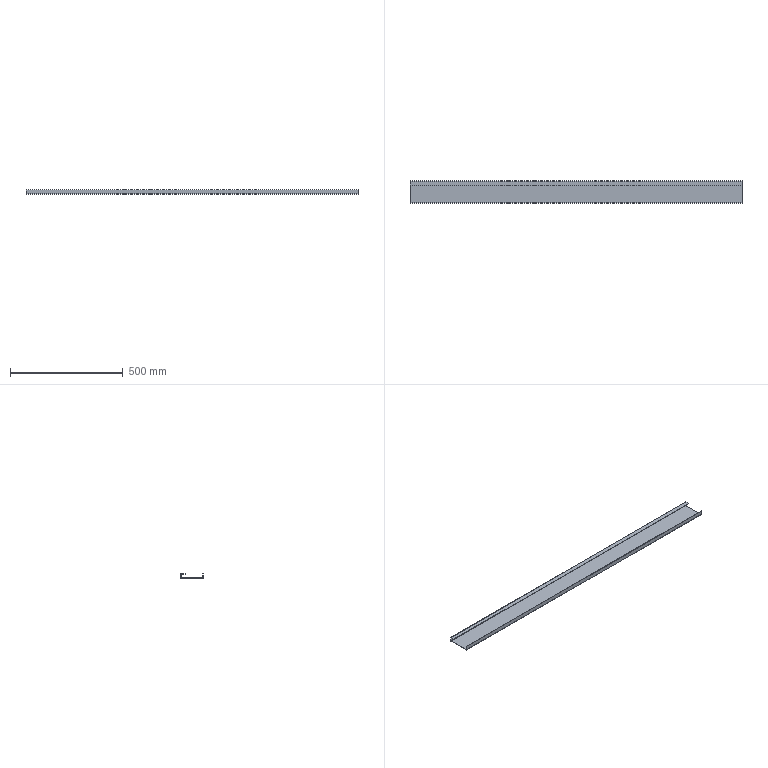Part | STEP file | 粉仓楼梯通道踢脚Plate 2 | 1 solid | 18 faces | box 1470 x 100 x 20 mm | volume 337909 mm3 | plane 12 | cylinder 6 | commonest cylinder face diameters 2 x3 5 x3
STEP:
#1=CARTESIAN_POINT('',(0.,0.,0.));
#2=DIRECTION('',(0.,0.,1.));
#3=DIRECTION('',(1.,0.,0.));
#4=AXIS2_PLACEMENT_3D('',#1,#2,#3);
#5=CARTESIAN_POINT('',(-735.,1.5,2.5));
#6=VERTEX_POINT('',#5);
#7=CARTESIAN_POINT('',(-735.,1.5,20.));
#8=VERTEX_POINT('',#7);
#9=CARTESIAN_POINT('',(-735.,1.5,2.5));
#10=DIRECTION('',(0.,0.,1.));
#11=VECTOR('',#10,1.);
#12=LINE('',#9,#11);
#13=CARTESIAN_POINT('',(735.,1.5,2.5));
#14=DIRECTION('',(0.,-1.,0.));
#15=DIRECTION('',(0.,0.,-1.));
#16=AXIS2_PLACEMENT_3D('',#13,#14,#15);
#17=PLANE('',#16);
#18=CARTESIAN_POINT('',(0.,-1470.));
#19=DIRECTION('',(-1.,0.));
#20=VECTOR('',#19,1.);
#21=LINE('',#18,#20);
#22=(GEOMETRIC_REPRESENTATION_CONTEXT(2)PARAMETRIC_REPRESENTATION_CONTEXT()REPRESENTATION_CONTEXT('',''));
#23=DEFINITIONAL_REPRESENTATION('',(#21),#22);
#24=PCURVE('',#17,#23);
#25=CARTESIAN_POINT('',(-735.,2.5,2.5));
#26=DIRECTION('',(-1.,0.,0.));
#27=DIRECTION('',(0.,0.,1.));
#28=AXIS2_PLACEMENT_3D('',#25,#26,#27);
#29=PLANE('',#28);
#30=CARTESIAN_POINT('',(0.,-1.));
#31=DIRECTION('',(1.,0.));
#32=VECTOR('',#31,1.);
#33=LINE('',#30,#32);
#34=(GEOMETRIC_REPRESENTATION_CONTEXT(2)PARAMETRIC_REPRESENTATION_CONTEXT()REPRESENTATION_CONTEXT('',''));
#35=DEFINITIONAL_REPRESENTATION('',(#33),#34);
#36=PCURVE('',#29,#35);
#37=SURFACE_CURVE('',#12,(#24,#36),.PCURVE_S1.);
#38=EDGE_CURVE('',#6,#8,#37,.T.);
#39=ORIENTED_EDGE('',*,*,#38,.T.);
#40=CARTESIAN_POINT('',(735.,1.5,20.));
#41=VERTEX_POINT('',#40);
#42=CARTESIAN_POINT('',(735.,1.5,20.));
#43=DIRECTION('',(-1.,0.,0.));
#44=VECTOR('',#43,1.);
#45=LINE('',#42,#44);
#46=CARTESIAN_POINT('',(-17.5,0.));
#47=DIRECTION('',(0.,-1.));
#48=VECTOR('',#47,1.);
#49=LINE('',#46,#48);
#50=(GEOMETRIC_REPRESENTATION_CONTEXT(2)PARAMETRIC_REPRESENTATION_CONTEXT()REPRESENTATION_CONTEXT('',''));
#51=DEFINITIONAL_REPRESENTATION('',(#49),#50);
#52=PCURVE('',#17,#51);
#53=CARTESIAN_POINT('',(735.,0.,20.));
#54=DIRECTION('',(0.,0.,1.));
#55=DIRECTION('',(1.,0.,0.));
#56=AXIS2_PLACEMENT_3D('',#53,#54,#55);
#57=PLANE('',#56);
#58=CARTESIAN_POINT('',(0.,1.5));
#59=DIRECTION('',(-1.,0.));
#60=VECTOR('',#59,1.);
#61=LINE('',#58,#60);
#62=(GEOMETRIC_REPRESENTATION_CONTEXT(2)PARAMETRIC_REPRESENTATION_CONTEXT()REPRESENTATION_CONTEXT('',''));
#63=DEFINITIONAL_REPRESENTATION('',(#61),#62);
#64=PCURVE('',#57,#63);
#65=SURFACE_CURVE('',#45,(#52,#64),.PCURVE_S1.);
#66=EDGE_CURVE('',#41,#8,#65,.T.);
#67=ORIENTED_EDGE('',*,*,#66,.F.);
#68=CARTESIAN_POINT('',(735.,1.5,2.5));
#69=VERTEX_POINT('',#68);
#70=CARTESIAN_POINT('',(735.,1.5,2.5));
#71=DIRECTION('',(0.,0.,1.));
#72=VECTOR('',#71,1.);
#73=LINE('',#70,#72);
#74=CARTESIAN_POINT('',(0.,0.));
#75=DIRECTION('',(-1.,0.));
#76=VECTOR('',#75,1.);
#77=LINE('',#74,#76);
#78=(GEOMETRIC_REPRESENTATION_CONTEXT(2)PARAMETRIC_REPRESENTATION_CONTEXT()REPRESENTATION_CONTEXT('',''));
#79=DEFINITIONAL_REPRESENTATION('',(#77),#78);
#80=PCURVE('',#17,#79);
#81=CARTESIAN_POINT('',(735.,2.5,2.5));
#82=DIRECTION('',(-1.,0.,0.));
#83=DIRECTION('',(0.,0.,1.));
#84=AXIS2_PLACEMENT_3D('',#81,#82,#83);
#85=PLANE('',#84);
#86=CARTESIAN_POINT('',(0.,-1.));
#87=DIRECTION('',(1.,0.));
#88=VECTOR('',#87,1.);
#89=LINE('',#86,#88);
#90=(GEOMETRIC_REPRESENTATION_CONTEXT(2)PARAMETRIC_REPRESENTATION_CONTEXT()REPRESENTATION_CONTEXT('',''));
#91=DEFINITIONAL_REPRESENTATION('',(#89),#90);
#92=PCURVE('',#85,#91);
#93=SURFACE_CURVE('',#73,(#80,#92),.PCURVE_S1.);
#94=EDGE_CURVE('',#69,#41,#93,.T.);
#95=ORIENTED_EDGE('',*,*,#94,.F.);
#96=CARTESIAN_POINT('',(735.,1.5,2.5));
#97=DIRECTION('',(-1.,0.,0.));
#98=VECTOR('',#97,1.);
#99=LINE('',#96,#98);
#100=CARTESIAN_POINT('',(0.,0.));
#101=DIRECTION('',(0.,-1.));
#102=VECTOR('',#101,1.);
#103=LINE('',#100,#102);
#104=(GEOMETRIC_REPRESENTATION_CONTEXT(2)PARAMETRIC_REPRESENTATION_CONTEXT()REPRESENTATION_CONTEXT('',''));
#105=DEFINITIONAL_REPRESENTATION('',(#103),#104);
#106=PCURVE('',#17,#105);
#107=CARTESIAN_POINT('',(735.,2.5,2.5));
#108=DIRECTION('',(-1.,0.,0.));
#109=DIRECTION('',(0.,0.,1.));
#110=AXIS2_PLACEMENT_3D('',#107,#108,#109);
#111=CYLINDRICAL_SURFACE('',#110,1.);
#112=CARTESIAN_POINT('',(4.712,0.));
#113=DIRECTION('',(0.,1.));
#114=VECTOR('',#113,1.);
#115=LINE('',#112,#114);
#116=(GEOMETRIC_REPRESENTATION_CONTEXT(2)PARAMETRIC_REPRESENTATION_CONTEXT()REPRESENTATION_CONTEXT('',''));
#117=DEFINITIONAL_REPRESENTATION('',(#115),#116);
#118=PCURVE('',#111,#117);
#119=SURFACE_CURVE('',#99,(#106,#118),.PCURVE_S1.);
#120=EDGE_CURVE('',#69,#6,#119,.T.);
#121=ORIENTED_EDGE('',*,*,#120,.T.);
#122=EDGE_LOOP('',(#39,#67,#95,#121));
#123=FACE_BOUND('',#122,.T.);
#124=ADVANCED_FACE('',(#123),#17,.F.);
#125=CARTESIAN_POINT('',(-735.,0.,20.));
#126=VERTEX_POINT('',#125);
#127=CARTESIAN_POINT('',(-735.,0.,20.));
#128=DIRECTION('',(0.,1.,0.));
#129=VECTOR('',#128,1.);
#130=LINE('',#127,#129);
#131=CARTESIAN_POINT('',(-1470.,0.));
#132=DIRECTION('',(0.,1.));
#133=VECTOR('',#132,1.);
#134=LINE('',#131,#133);
#135=(GEOMETRIC_REPRESENTATION_CONTEXT(2)PARAMETRIC_REPRESENTATION_CONTEXT()REPRESENTATION_CONTEXT('',''));
#136=DEFINITIONAL_REPRESENTATION('',(#134),#135);
#137=PCURVE('',#57,#136);
#138=CARTESIAN_POINT('',(17.5,-2.5));
#139=DIRECTION('',(0.,1.));
#140=VECTOR('',#139,1.);
#141=LINE('',#138,#140);
#142=(GEOMETRIC_REPRESENTATION_CONTEXT(2)PARAMETRIC_REPRESENTATION_CONTEXT()REPRESENTATION_CONTEXT('',''));
#143=DEFINITIONAL_REPRESENTATION('',(#141),#142);
#144=PCURVE('',#29,#143);
#145=SURFACE_CURVE('',#130,(#137,#144),.PCURVE_S1.);
#146=EDGE_CURVE('',#126,#8,#145,.T.);
#147=ORIENTED_EDGE('',*,*,#146,.F.);
#148=CARTESIAN_POINT('',(735.,0.,20.));
#149=VERTEX_POINT('',#148);
#150=CARTESIAN_POINT('',(735.,0.,20.));
#151=DIRECTION('',(-1.,0.,0.));
#152=VECTOR('',#151,1.);
#153=LINE('',#150,#152);
#154=CARTESIAN_POINT('',(0.,0.));
#155=DIRECTION('',(-1.,0.));
#156=VECTOR('',#155,1.);
#157=LINE('',#154,#156);
#158=(GEOMETRIC_REPRESENTATION_CONTEXT(2)PARAMETRIC_REPRESENTATION_CONTEXT()REPRESENTATION_CONTEXT('',''));
#159=DEFINITIONAL_REPRESENTATION('',(#157),#158);
#160=PCURVE('',#57,#159);
#161=CARTESIAN_POINT('',(735.,0.,2.5));
#162=DIRECTION('',(0.,-1.,0.));
#163=DIRECTION('',(0.,0.,-1.));
#164=AXIS2_PLACEMENT_3D('',#161,#162,#163);
#165=PLANE('',#164);
#166=CARTESIAN_POINT('',(-17.5,0.));
#167=DIRECTION('',(0.,-1.));
#168=VECTOR('',#167,1.);
#169=LINE('',#166,#168);
#170=(GEOMETRIC_REPRESENTATION_CONTEXT(2)PARAMETRIC_REPRESENTATION_CONTEXT()REPRESENTATION_CONTEXT('',''));
#171=DEFINITIONAL_REPRESENTATION('',(#169),#170);
#172=PCURVE('',#165,#171);
#173=SURFACE_CURVE('',#153,(#160,#172),.PCURVE_S1.);
#174=EDGE_CURVE('',#149,#126,#173,.T.);
#175=ORIENTED_EDGE('',*,*,#174,.F.);
#176=CARTESIAN_POINT('',(735.,0.,20.));
#177=DIRECTION('',(0.,1.,0.));
#178=VECTOR('',#177,1.);
#179=LINE('',#176,#178);
#180=CARTESIAN_POINT('',(0.,0.));
#181=DIRECTION('',(0.,1.));
#182=VECTOR('',#181,1.);
#183=LINE('',#180,#182);
#184=(GEOMETRIC_REPRESENTATION_CONTEXT(2)PARAMETRIC_REPRESENTATION_CONTEXT()REPRESENTATION_CONTEXT('',''));
#185=DEFINITIONAL_REPRESENTATION('',(#183),#184);
#186=PCURVE('',#57,#185);
#187=CARTESIAN_POINT('',(17.5,-2.5));
#188=DIRECTION('',(0.,1.));
#189=VECTOR('',#188,1.);
#190=LINE('',#187,#189);
#191=(GEOMETRIC_REPRESENTATION_CONTEXT(2)PARAMETRIC_REPRESENTATION_CONTEXT()REPRESENTATION_CONTEXT('',''));
#192=DEFINITIONAL_REPRESENTATION('',(#190),#191);
#193=PCURVE('',#85,#192);
#194=SURFACE_CURVE('',#179,(#186,#193),.PCURVE_S1.);
#195=EDGE_CURVE('',#149,#41,#194,.T.);
#196=ORIENTED_EDGE('',*,*,#195,.T.);
#197=ORIENTED_EDGE('',*,*,#66,.T.);
#198=EDGE_LOOP('',(#147,#175,#196,#197));
#199=FACE_BOUND('',#198,.T.);
#200=ADVANCED_FACE('',(#199),#57,.T.);
#201=CARTESIAN_POINT('',(-735.,0.,2.5));
#202=VERTEX_POINT('',#201);
#203=CARTESIAN_POINT('',(-735.,0.,2.5));
#204=DIRECTION('',(0.,0.,1.));
#205=VECTOR('',#204,1.);
#206=LINE('',#203,#205);
#207=CARTESIAN_POINT('',(0.,-1470.));
#208=DIRECTION('',(-1.,0.));
#209=VECTOR('',#208,1.);
#210=LINE('',#207,#209);
#211=(GEOMETRIC_REPRESENTATION_CONTEXT(2)PARAMETRIC_REPRESENTATION_CONTEXT()REPRESENTATION_CONTEXT('',''));
#212=DEFINITIONAL_REPRESENTATION('',(#210),#211);
#213=PCURVE('',#165,#212);
#214=CARTESIAN_POINT('',(0.,-2.5));
#215=DIRECTION('',(1.,0.));
#216=VECTOR('',#215,1.);
#217=LINE('',#214,#216);
#218=(GEOMETRIC_REPRESENTATION_CONTEXT(2)PARAMETRIC_REPRESENTATION_CONTEXT()REPRESENTATION_CONTEXT('',''));
#219=DEFINITIONAL_REPRESENTATION('',(#217),#218);
#220=PCURVE('',#29,#219);
#221=SURFACE_CURVE('',#206,(#213,#220),.PCURVE_S1.);
#222=EDGE_CURVE('',#202,#126,#221,.T.);
#223=ORIENTED_EDGE('',*,*,#222,.F.);
#224=CARTESIAN_POINT('',(735.,0.,2.5));
#225=VERTEX_POINT('',#224);
#226=CARTESIAN_POINT('',(735.,0.,2.5));
#227=DIRECTION('',(-1.,0.,0.));
#228=VECTOR('',#227,1.);
#229=LINE('',#226,#228);
#230=CARTESIAN_POINT('',(0.,0.));
#231=DIRECTION('',(0.,-1.));
#232=VECTOR('',#231,1.);
#233=LINE('',#230,#232);
#234=(GEOMETRIC_REPRESENTATION_CONTEXT(2)PARAMETRIC_REPRESENTATION_CONTEXT()REPRESENTATION_CONTEXT('',''));
#235=DEFINITIONAL_REPRESENTATION('',(#233),#234);
#236=PCURVE('',#165,#235);
#237=CARTESIAN_POINT('',(735.,2.5,2.5));
#238=DIRECTION('',(-1.,0.,0.));
#239=DIRECTION('',(0.,0.,1.));
#240=AXIS2_PLACEMENT_3D('',#237,#238,#239);
#241=CYLINDRICAL_SURFACE('',#240,2.5);
#242=CARTESIAN_POINT('',(4.712,0.));
#243=DIRECTION('',(0.,1.));
#244=VECTOR('',#243,1.);
#245=LINE('',#242,#244);
#246=(GEOMETRIC_REPRESENTATION_CONTEXT(2)PARAMETRIC_REPRESENTATION_CONTEXT()REPRESENTATION_CONTEXT('',''));
#247=DEFINITIONAL_REPRESENTATION('',(#245),#246);
#248=PCURVE('',#241,#247);
#249=SURFACE_CURVE('',#229,(#236,#248),.PCURVE_S1.);
#250=EDGE_CURVE('',#225,#202,#249,.T.);
#251=ORIENTED_EDGE('',*,*,#250,.F.);
#252=CARTESIAN_POINT('',(735.,0.,2.5));
#253=DIRECTION('',(0.,0.,1.));
#254=VECTOR('',#253,1.);
#255=LINE('',#252,#254);
#256=CARTESIAN_POINT('',(0.,0.));
#257=DIRECTION('',(-1.,0.));
#258=VECTOR('',#257,1.);
#259=LINE('',#256,#258);
#260=(GEOMETRIC_REPRESENTATION_CONTEXT(2)PARAMETRIC_REPRESENTATION_CONTEXT()REPRESENTATION_CONTEXT('',''));
#261=DEFINITIONAL_REPRESENTATION('',(#259),#260);
#262=PCURVE('',#165,#261);
#263=CARTESIAN_POINT('',(0.,-2.5));
#264=DIRECTION('',(1.,0.));
#265=VECTOR('',#264,1.);
#266=LINE('',#263,#265);
#267=(GEOMETRIC_REPRESENTATION_CONTEXT(2)PARAMETRIC_REPRESENTATION_CONTEXT()REPRESENTATION_CONTEXT('',''));
#268=DEFINITIONAL_REPRESENTATION('',(#266),#267);
#269=PCURVE('',#85,#268);
#270=SURFACE_CURVE('',#255,(#262,#269),.PCURVE_S1.);
#271=EDGE_CURVE('',#225,#149,#270,.T.);
#272=ORIENTED_EDGE('',*,*,#271,.T.);
#273=ORIENTED_EDGE('',*,*,#174,.T.);
#274=EDGE_LOOP('',(#223,#251,#272,#273));
#275=FACE_BOUND('',#274,.T.);
#276=ADVANCED_FACE('',(#275),#165,.T.);
#277=CARTESIAN_POINT('',(-735.,2.5,0.));
#278=VERTEX_POINT('',#277);
#279=CARTESIAN_POINT('',(-735.,2.5,2.5));
#280=DIRECTION('',(-1.,0.,0.));
#281=DIRECTION('',(0.,0.,1.));
#282=AXIS2_PLACEMENT_3D('',#279,#280,#281);
#283=CIRCLE('',#282,2.5);
#284=CARTESIAN_POINT('',(0.,1470.));
#285=DIRECTION('',(1.,0.));
#286=VECTOR('',#285,1.);
#287=LINE('',#284,#286);
#288=(GEOMETRIC_REPRESENTATION_CONTEXT(2)PARAMETRIC_REPRESENTATION_CONTEXT()REPRESENTATION_CONTEXT('',''));
#289=DEFINITIONAL_REPRESENTATION('',(#287),#288);
#290=PCURVE('',#241,#289);
#291=CARTESIAN_POINT('',(0.,0.));
#292=DIRECTION('',(1.,0.));
#293=AXIS2_PLACEMENT_2D('',#291,#292);
#294=CIRCLE('',#293,2.5);
#295=(GEOMETRIC_REPRESENTATION_CONTEXT(2)PARAMETRIC_REPRESENTATION_CONTEXT()REPRESENTATION_CONTEXT('',''));
#296=DEFINITIONAL_REPRESENTATION('',(#294),#295);
#297=PCURVE('',#29,#296);
#298=SURFACE_CURVE('',#283,(#290,#297),.PCURVE_S1.);
#299=EDGE_CURVE('',#278,#202,#298,.T.);
#300=ORIENTED_EDGE('',*,*,#299,.F.);
#301=CARTESIAN_POINT('',(735.,2.5,0.));
#302=VERTEX_POINT('',#301);
#303=CARTESIAN_POINT('',(735.,2.5,0.));
#304=DIRECTION('',(-1.,0.,0.));
#305=VECTOR('',#304,1.);
#306=LINE('',#303,#305);
#307=CARTESIAN_POINT('',(3.142,0.));
#308=DIRECTION('',(0.,1.));
#309=VECTOR('',#308,1.);
#310=LINE('',#307,#309);
#311=(GEOMETRIC_REPRESENTATION_CONTEXT(2)PARAMETRIC_REPRESENTATION_CONTEXT()REPRESENTATION_CONTEXT('',''));
#312=DEFINITIONAL_REPRESENTATION('',(#310),#311);
#313=PCURVE('',#241,#312);
#314=CARTESIAN_POINT('',(735.,2.5,0.));
#315=DIRECTION('',(0.,0.,-1.));
#316=DIRECTION('',(-1.,0.,0.));
#317=AXIS2_PLACEMENT_3D('',#314,#315,#316);
#318=PLANE('',#317);
#319=CARTESIAN_POINT('',(0.,0.));
#320=DIRECTION('',(1.,0.));
#321=VECTOR('',#320,1.);
#322=LINE('',#319,#321);
#323=(GEOMETRIC_REPRESENTATION_CONTEXT(2)PARAMETRIC_REPRESENTATION_CONTEXT()REPRESENTATION_CONTEXT('',''));
#324=DEFINITIONAL_REPRESENTATION('',(#322),#323);
#325=PCURVE('',#318,#324);
#326=SURFACE_CURVE('',#306,(#313,#325),.PCURVE_S1.);
#327=EDGE_CURVE('',#302,#278,#326,.T.);
#328=ORIENTED_EDGE('',*,*,#327,.F.);
#329=CARTESIAN_POINT('',(735.,2.5,2.5));
#330=DIRECTION('',(-1.,0.,0.));
#331=DIRECTION('',(0.,0.,1.));
#332=AXIS2_PLACEMENT_3D('',#329,#330,#331);
#333=CIRCLE('',#332,2.5);
#334=CARTESIAN_POINT('',(0.,0.));
#335=DIRECTION('',(1.,0.));
#336=VECTOR('',#335,1.);
#337=LINE('',#334,#336);
#338=(GEOMETRIC_REPRESENTATION_CONTEXT(2)PARAMETRIC_REPRESENTATION_CONTEXT()REPRESENTATION_CONTEXT('',''));
#339=DEFINITIONAL_REPRESENTATION('',(#337),#338);
#340=PCURVE('',#241,#339);
#341=CARTESIAN_POINT('',(0.,0.));
#342=DIRECTION('',(1.,0.));
#343=AXIS2_PLACEMENT_2D('',#341,#342);
#344=CIRCLE('',#343,2.5);
#345=(GEOMETRIC_REPRESENTATION_CONTEXT(2)PARAMETRIC_REPRESENTATION_CONTEXT()REPRESENTATION_CONTEXT('',''));
#346=DEFINITIONAL_REPRESENTATION('',(#344),#345);
#347=PCURVE('',#85,#346);
#348=SURFACE_CURVE('',#333,(#340,#347),.PCURVE_S1.);
#349=EDGE_CURVE('',#302,#225,#348,.T.);
#350=ORIENTED_EDGE('',*,*,#349,.T.);
#351=ORIENTED_EDGE('',*,*,#250,.T.);
#352=EDGE_LOOP('',(#300,#328,#350,#351));
#353=FACE_BOUND('',#352,.T.);
#354=ADVANCED_FACE('',(#353),#241,.T.);
#355=CARTESIAN_POINT('',(-735.,97.5,0.));
#356=VERTEX_POINT('',#355);
#357=CARTESIAN_POINT('',(-735.,2.5,0.));
#358=DIRECTION('',(0.,-1.,0.));
#359=VECTOR('',#358,1.);
#360=LINE('',#357,#359);
#361=CARTESIAN_POINT('',(1470.,0.));
#362=DIRECTION('',(0.,-1.));
#363=VECTOR('',#362,1.);
#364=LINE('',#361,#363);
#365=(GEOMETRIC_REPRESENTATION_CONTEXT(2)PARAMETRIC_REPRESENTATION_CONTEXT()REPRESENTATION_CONTEXT('',''));
#366=DEFINITIONAL_REPRESENTATION('',(#364),#365);
#367=PCURVE('',#318,#366);
#368=CARTESIAN_POINT('',(-2.5,0.));
#369=DIRECTION('',(0.,-1.));
#370=VECTOR('',#369,1.);
#371=LINE('',#368,#370);
#372=(GEOMETRIC_REPRESENTATION_CONTEXT(2)PARAMETRIC_REPRESENTATION_CONTEXT()REPRESENTATION_CONTEXT('',''));
#373=DEFINITIONAL_REPRESENTATION('',(#371),#372);
#374=PCURVE('',#29,#373);
#375=SURFACE_CURVE('',#360,(#367,#374),.PCURVE_S1.);
#376=EDGE_CURVE('',#356,#278,#375,.T.);
#377=ORIENTED_EDGE('',*,*,#376,.F.);
#378=CARTESIAN_POINT('',(735.,97.5,0.));
#379=VERTEX_POINT('',#378);
#380=CARTESIAN_POINT('',(735.,97.5,0.));
#381=DIRECTION('',(-1.,0.,0.));
#382=VECTOR('',#381,1.);
#383=LINE('',#380,#382);
#384=CARTESIAN_POINT('',(0.,95.));
#385=DIRECTION('',(1.,0.));
#386=VECTOR('',#385,1.);
#387=LINE('',#384,#386);
#388=(GEOMETRIC_REPRESENTATION_CONTEXT(2)PARAMETRIC_REPRESENTATION_CONTEXT()REPRESENTATION_CONTEXT('',''));
#389=DEFINITIONAL_REPRESENTATION('',(#387),#388);
#390=PCURVE('',#318,#389);
#391=CARTESIAN_POINT('',(735.,97.5,2.5));
#392=DIRECTION('',(-1.,0.,0.));
#393=DIRECTION('',(0.,0.,1.));
#394=AXIS2_PLACEMENT_3D('',#391,#392,#393);
#395=CYLINDRICAL_SURFACE('',#394,2.5);
#396=CARTESIAN_POINT('',(3.142,0.));
#397=DIRECTION('',(0.,1.));
#398=VECTOR('',#397,1.);
#399=LINE('',#396,#398);
#400=(GEOMETRIC_REPRESENTATION_CONTEXT(2)PARAMETRIC_REPRESENTATION_CONTEXT()REPRESENTATION_CONTEXT('',''));
#401=DEFINITIONAL_REPRESENTATION('',(#399),#400);
#402=PCURVE('',#395,#401);
#403=SURFACE_CURVE('',#383,(#390,#402),.PCURVE_S1.);
#404=EDGE_CURVE('',#379,#356,#403,.T.);
#405=ORIENTED_EDGE('',*,*,#404,.F.);
#406=CARTESIAN_POINT('',(735.,2.5,0.));
#407=DIRECTION('',(0.,-1.,0.));
#408=VECTOR('',#407,1.);
#409=LINE('',#406,#408);
#410=CARTESIAN_POINT('',(0.,0.));
#411=DIRECTION('',(0.,-1.));
#412=VECTOR('',#411,1.);
#413=LINE('',#410,#412);
#414=(GEOMETRIC_REPRESENTATION_CONTEXT(2)PARAMETRIC_REPRESENTATION_CONTEXT()REPRESENTATION_CONTEXT('',''));
#415=DEFINITIONAL_REPRESENTATION('',(#413),#414);
#416=PCURVE('',#318,#415);
#417=CARTESIAN_POINT('',(-2.5,0.));
#418=DIRECTION('',(0.,-1.));
#419=VECTOR('',#418,1.);
#420=LINE('',#417,#419);
#421=(GEOMETRIC_REPRESENTATION_CONTEXT(2)PARAMETRIC_REPRESENTATION_CONTEXT()REPRESENTATION_CONTEXT('',''));
#422=DEFINITIONAL_REPRESENTATION('',(#420),#421);
#423=PCURVE('',#85,#422);
#424=SURFACE_CURVE('',#409,(#416,#423),.PCURVE_S1.);
#425=EDGE_CURVE('',#379,#302,#424,.T.);
#426=ORIENTED_EDGE('',*,*,#425,.T.);
#427=ORIENTED_EDGE('',*,*,#327,.T.);
#428=EDGE_LOOP('',(#377,#405,#426,#427));
#429=FACE_BOUND('',#428,.T.);
#430=ADVANCED_FACE('',(#429),#318,.T.);
#431=CARTESIAN_POINT('',(-735.,100.,2.5));
#432=VERTEX_POINT('',#431);
#433=CARTESIAN_POINT('',(-735.,97.5,2.5));
#434=DIRECTION('',(-1.,0.,0.));
#435=DIRECTION('',(0.,0.,-1.));
#436=AXIS2_PLACEMENT_3D('',#433,#434,#435);
#437=CIRCLE('',#436,2.5);
#438=CARTESIAN_POINT('',(-3.142,1470.));
#439=DIRECTION('',(1.,0.));
#440=VECTOR('',#439,1.);
#441=LINE('',#438,#440);
#442=(GEOMETRIC_REPRESENTATION_CONTEXT(2)PARAMETRIC_REPRESENTATION_CONTEXT()REPRESENTATION_CONTEXT('',''));
#443=DEFINITIONAL_REPRESENTATION('',(#441),#442);
#444=PCURVE('',#395,#443);
#445=CARTESIAN_POINT('',(0.,95.));
#446=DIRECTION('',(-1.,0.));
#447=AXIS2_PLACEMENT_2D('',#445,#446);
#448=CIRCLE('',#447,2.5);
#449=(GEOMETRIC_REPRESENTATION_CONTEXT(2)PARAMETRIC_REPRESENTATION_CONTEXT()REPRESENTATION_CONTEXT('',''));
#450=DEFINITIONAL_REPRESENTATION('',(#448),#449);
#451=PCURVE('',#29,#450);
#452=SURFACE_CURVE('',#437,(#444,#451),.PCURVE_S1.);
#453=EDGE_CURVE('',#432,#356,#452,.T.);
#454=ORIENTED_EDGE('',*,*,#453,.F.);
#455=CARTESIAN_POINT('',(735.,100.,2.5));
#456=VERTEX_POINT('',#455);
#457=CARTESIAN_POINT('',(735.,100.,2.5));
#458=DIRECTION('',(-1.,0.,0.));
#459=VECTOR('',#458,1.);
#460=LINE('',#457,#459);
#461=CARTESIAN_POINT('',(1.571,0.));
#462=DIRECTION('',(0.,1.));
#463=VECTOR('',#462,1.);
#464=LINE('',#461,#463);
#465=(GEOMETRIC_REPRESENTATION_CONTEXT(2)PARAMETRIC_REPRESENTATION_CONTEXT()REPRESENTATION_CONTEXT('',''));
#466=DEFINITIONAL_REPRESENTATION('',(#464),#465);
#467=PCURVE('',#395,#466);
#468=CARTESIAN_POINT('',(735.,100.,2.5));
#469=DIRECTION('',(0.,1.,0.));
#470=DIRECTION('',(0.,0.,1.));
#471=AXIS2_PLACEMENT_3D('',#468,#469,#470);
#472=PLANE('',#471);
#473=CARTESIAN_POINT('',(0.,0.));
#474=DIRECTION('',(0.,-1.));
#475=VECTOR('',#474,1.);
#476=LINE('',#473,#475);
#477=(GEOMETRIC_REPRESENTATION_CONTEXT(2)PARAMETRIC_REPRESENTATION_CONTEXT()REPRESENTATION_CONTEXT('',''));
#478=DEFINITIONAL_REPRESENTATION('',(#476),#477);
#479=PCURVE('',#472,#478);
#480=SURFACE_CURVE('',#460,(#467,#479),.PCURVE_S1.);
#481=EDGE_CURVE('',#456,#432,#480,.T.);
#482=ORIENTED_EDGE('',*,*,#481,.F.);
#483=CARTESIAN_POINT('',(735.,97.5,2.5));
#484=DIRECTION('',(-1.,0.,0.));
#485=DIRECTION('',(0.,0.,-1.));
#486=AXIS2_PLACEMENT_3D('',#483,#484,#485);
#487=CIRCLE('',#486,2.5);
#488=CARTESIAN_POINT('',(-3.142,0.));
#489=DIRECTION('',(1.,0.));
#490=VECTOR('',#489,1.);
#491=LINE('',#488,#490);
#492=(GEOMETRIC_REPRESENTATION_CONTEXT(2)PARAMETRIC_REPRESENTATION_CONTEXT()REPRESENTATION_CONTEXT('',''));
#493=DEFINITIONAL_REPRESENTATION('',(#491),#492);
#494=PCURVE('',#395,#493);
#495=CARTESIAN_POINT('',(0.,95.));
#496=DIRECTION('',(-1.,0.));
#497=AXIS2_PLACEMENT_2D('',#495,#496);
#498=CIRCLE('',#497,2.5);
#499=(GEOMETRIC_REPRESENTATION_CONTEXT(2)PARAMETRIC_REPRESENTATION_CONTEXT()REPRESENTATION_CONTEXT('',''));
#500=DEFINITIONAL_REPRESENTATION('',(#498),#499);
#501=PCURVE('',#85,#500);
#502=SURFACE_CURVE('',#487,(#494,#501),.PCURVE_S1.);
#503=EDGE_CURVE('',#456,#379,#502,.T.);
#504=ORIENTED_EDGE('',*,*,#503,.T.);
#505=ORIENTED_EDGE('',*,*,#404,.T.);
#506=EDGE_LOOP('',(#454,#482,#504,#505));
#507=FACE_BOUND('',#506,.T.);
#508=ADVANCED_FACE('',(#507),#395,.T.);
#509=CARTESIAN_POINT('',(-735.,100.,17.5));
#510=VERTEX_POINT('',#509);
#511=CARTESIAN_POINT('',(-735.,100.,2.5));
#512=DIRECTION('',(0.,0.,-1.));
#513=VECTOR('',#512,1.);
#514=LINE('',#511,#513);
#515=CARTESIAN_POINT('',(0.,-1470.));
#516=DIRECTION('',(-1.,0.));
#517=VECTOR('',#516,1.);
#518=LINE('',#515,#517);
#519=(GEOMETRIC_REPRESENTATION_CONTEXT(2)PARAMETRIC_REPRESENTATION_CONTEXT()REPRESENTATION_CONTEXT('',''));
#520=DEFINITIONAL_REPRESENTATION('',(#518),#519);
#521=PCURVE('',#472,#520);
#522=CARTESIAN_POINT('',(0.,97.5));
#523=DIRECTION('',(-1.,0.));
#524=VECTOR('',#523,1.);
#525=LINE('',#522,#524);
#526=(GEOMETRIC_REPRESENTATION_CONTEXT(2)PARAMETRIC_REPRESENTATION_CONTEXT()REPRESENTATION_CONTEXT('',''));
#527=DEFINITIONAL_REPRESENTATION('',(#525),#526);
#528=PCURVE('',#29,#527);
#529=SURFACE_CURVE('',#514,(#521,#528),.PCURVE_S1.);
#530=EDGE_CURVE('',#510,#432,#529,.T.);
#531=ORIENTED_EDGE('',*,*,#530,.F.);
#532=CARTESIAN_POINT('',(735.,100.,17.5));
#533=VERTEX_POINT('',#532);
#534=CARTESIAN_POINT('',(735.,100.,17.5));
#535=DIRECTION('',(-1.,0.,0.));
#536=VECTOR('',#535,1.);
#537=LINE('',#534,#536);
#538=CARTESIAN_POINT('',(15.,0.));
#539=DIRECTION('',(0.,-1.));
#540=VECTOR('',#539,1.);
#541=LINE('',#538,#540);
#542=(GEOMETRIC_REPRESENTATION_CONTEXT(2)PARAMETRIC_REPRESENTATION_CONTEXT()REPRESENTATION_CONTEXT('',''));
#543=DEFINITIONAL_REPRESENTATION('',(#541),#542);
#544=PCURVE('',#472,#543);
#545=CARTESIAN_POINT('',(735.,97.5,17.5));
#546=DIRECTION('',(-1.,0.,0.));
#547=DIRECTION('',(0.,0.,1.));
#548=AXIS2_PLACEMENT_3D('',#545,#546,#547);
#549=CYLINDRICAL_SURFACE('',#548,2.5);
#550=CARTESIAN_POINT('',(1.571,0.));
#551=DIRECTION('',(0.,1.));
#552=VECTOR('',#551,1.);
#553=LINE('',#550,#552);
#554=(GEOMETRIC_REPRESENTATION_CONTEXT(2)PARAMETRIC_REPRESENTATION_CONTEXT()REPRESENTATION_CONTEXT('',''));
#555=DEFINITIONAL_REPRESENTATION('',(#553),#554);
#556=PCURVE('',#549,#555);
#557=SURFACE_CURVE('',#537,(#544,#556),.PCURVE_S1.);
#558=EDGE_CURVE('',#533,#510,#557,.T.);
#559=ORIENTED_EDGE('',*,*,#558,.F.);
#560=CARTESIAN_POINT('',(735.,100.,2.5));
#561=DIRECTION('',(0.,0.,-1.));
#562=VECTOR('',#561,1.);
#563=LINE('',#560,#562);
#564=CARTESIAN_POINT('',(0.,0.));
#565=DIRECTION('',(-1.,0.));
#566=VECTOR('',#565,1.);
#567=LINE('',#564,#566);
#568=(GEOMETRIC_REPRESENTATION_CONTEXT(2)PARAMETRIC_REPRESENTATION_CONTEXT()REPRESENTATION_CONTEXT('',''));
#569=DEFINITIONAL_REPRESENTATION('',(#567),#568);
#570=PCURVE('',#472,#569);
#571=CARTESIAN_POINT('',(0.,97.5));
#572=DIRECTION('',(-1.,0.));
#573=VECTOR('',#572,1.);
#574=LINE('',#571,#573);
#575=(GEOMETRIC_REPRESENTATION_CONTEXT(2)PARAMETRIC_REPRESENTATION_CONTEXT()REPRESENTATION_CONTEXT('',''));
#576=DEFINITIONAL_REPRESENTATION('',(#574),#575);
#577=PCURVE('',#85,#576);
#578=SURFACE_CURVE('',#563,(#570,#577),.PCURVE_S1.);
#579=EDGE_CURVE('',#533,#456,#578,.T.);
#580=ORIENTED_EDGE('',*,*,#579,.T.);
#581=ORIENTED_EDGE('',*,*,#481,.T.);
#582=EDGE_LOOP('',(#531,#559,#580,#581));
#583=FACE_BOUND('',#582,.T.);
#584=ADVANCED_FACE('',(#583),#472,.T.);
#585=CARTESIAN_POINT('',(-735.,97.5,20.));
#586=VERTEX_POINT('',#585);
#587=CARTESIAN_POINT('',(-735.,97.5,17.5));
#588=DIRECTION('',(-1.,0.,0.));
#589=DIRECTION('',(0.,0.,-1.));
#590=AXIS2_PLACEMENT_3D('',#587,#588,#589);
#591=CIRCLE('',#590,2.5);
#592=CARTESIAN_POINT('',(-3.142,1470.));
#593=DIRECTION('',(1.,0.));
#594=VECTOR('',#593,1.);
#595=LINE('',#592,#594);
#596=(GEOMETRIC_REPRESENTATION_CONTEXT(2)PARAMETRIC_REPRESENTATION_CONTEXT()REPRESENTATION_CONTEXT('',''));
#597=DEFINITIONAL_REPRESENTATION('',(#595),#596);
#598=PCURVE('',#549,#597);
#599=CARTESIAN_POINT('',(15.,95.));
#600=DIRECTION('',(-1.,0.));
#601=AXIS2_PLACEMENT_2D('',#599,#600);
#602=CIRCLE('',#601,2.5);
#603=(GEOMETRIC_REPRESENTATION_CONTEXT(2)PARAMETRIC_REPRESENTATION_CONTEXT()REPRESENTATION_CONTEXT('',''));
#604=DEFINITIONAL_REPRESENTATION('',(#602),#603);
#605=PCURVE('',#29,#604);
#606=SURFACE_CURVE('',#591,(#598,#605),.PCURVE_S1.);
#607=EDGE_CURVE('',#586,#510,#606,.T.);
#608=ORIENTED_EDGE('',*,*,#607,.F.);
#609=CARTESIAN_POINT('',(735.,97.5,20.));
#610=VERTEX_POINT('',#609);
#611=CARTESIAN_POINT('',(735.,97.5,20.));
#612=DIRECTION('',(-1.,0.,0.));
#613=VECTOR('',#612,1.);
#614=LINE('',#611,#613);
#615=CARTESIAN_POINT('',(0.,0.));
#616=DIRECTION('',(0.,1.));
#617=VECTOR('',#616,1.);
#618=LINE('',#615,#617);
#619=(GEOMETRIC_REPRESENTATION_CONTEXT(2)PARAMETRIC_REPRESENTATION_CONTEXT()REPRESENTATION_CONTEXT('',''));
#620=DEFINITIONAL_REPRESENTATION('',(#618),#619);
#621=PCURVE('',#549,#620);
#622=CARTESIAN_POINT('',(735.,97.5,20.));
#623=DIRECTION('',(0.,0.,1.));
#624=DIRECTION('',(1.,0.,0.));
#625=AXIS2_PLACEMENT_3D('',#622,#623,#624);
#626=PLANE('',#625);
#627=CARTESIAN_POINT('',(0.,0.));
#628=DIRECTION('',(-1.,0.));
#629=VECTOR('',#628,1.);
#630=LINE('',#627,#629);
#631=(GEOMETRIC_REPRESENTATION_CONTEXT(2)PARAMETRIC_REPRESENTATION_CONTEXT()REPRESENTATION_CONTEXT('',''));
#632=DEFINITIONAL_REPRESENTATION('',(#630),#631);
#633=PCURVE('',#626,#632);
#634=SURFACE_CURVE('',#614,(#621,#633),.PCURVE_S1.);
#635=EDGE_CURVE('',#610,#586,#634,.T.);
#636=ORIENTED_EDGE('',*,*,#635,.F.);
#637=CARTESIAN_POINT('',(735.,97.5,17.5));
#638=DIRECTION('',(-1.,0.,0.));
#639=DIRECTION('',(0.,0.,-1.));
#640=AXIS2_PLACEMENT_3D('',#637,#638,#639);
#641=CIRCLE('',#640,2.5);
#642=CARTESIAN_POINT('',(-3.142,0.));
#643=DIRECTION('',(1.,0.));
#644=VECTOR('',#643,1.);
#645=LINE('',#642,#644);
#646=(GEOMETRIC_REPRESENTATION_CONTEXT(2)PARAMETRIC_REPRESENTATION_CONTEXT()REPRESENTATION_CONTEXT('',''));
#647=DEFINITIONAL_REPRESENTATION('',(#645),#646);
#648=PCURVE('',#549,#647);
#649=CARTESIAN_POINT('',(15.,95.));
#650=DIRECTION('',(-1.,0.));
#651=AXIS2_PLACEMENT_2D('',#649,#650);
#652=CIRCLE('',#651,2.5);
#653=(GEOMETRIC_REPRESENTATION_CONTEXT(2)PARAMETRIC_REPRESENTATION_CONTEXT()REPRESENTATION_CONTEXT('',''));
#654=DEFINITIONAL_REPRESENTATION('',(#652),#653);
#655=PCURVE('',#85,#654);
#656=SURFACE_CURVE('',#641,(#648,#655),.PCURVE_S1.);
#657=EDGE_CURVE('',#610,#533,#656,.T.);
#658=ORIENTED_EDGE('',*,*,#657,.T.);
#659=ORIENTED_EDGE('',*,*,#558,.T.);
#660=EDGE_LOOP('',(#608,#636,#658,#659));
#661=FACE_BOUND('',#660,.T.);
#662=ADVANCED_FACE('',(#661),#549,.T.);
#663=CARTESIAN_POINT('',(-735.,80.,20.));
#664=VERTEX_POINT('',#663);
#665=CARTESIAN_POINT('',(-735.,97.5,20.));
#666=DIRECTION('',(0.,1.,0.));
#667=VECTOR('',#666,1.);
#668=LINE('',#665,#667);
#669=CARTESIAN_POINT('',(-1470.,0.));
#670=DIRECTION('',(0.,1.));
#671=VECTOR('',#670,1.);
#672=LINE('',#669,#671);
#673=(GEOMETRIC_REPRESENTATION_CONTEXT(2)PARAMETRIC_REPRESENTATION_CONTEXT()REPRESENTATION_CONTEXT('',''));
#674=DEFINITIONAL_REPRESENTATION('',(#672),#673);
#675=PCURVE('',#626,#674);
#676=CARTESIAN_POINT('',(17.5,95.));
#677=DIRECTION('',(0.,1.));
#678=VECTOR('',#677,1.);
#679=LINE('',#676,#678);
#680=(GEOMETRIC_REPRESENTATION_CONTEXT(2)PARAMETRIC_REPRESENTATION_CONTEXT()REPRESENTATION_CONTEXT('',''));
#681=DEFINITIONAL_REPRESENTATION('',(#679),#680);
#682=PCURVE('',#29,#681);
#683=SURFACE_CURVE('',#668,(#675,#682),.PCURVE_S1.);
#684=EDGE_CURVE('',#664,#586,#683,.T.);
#685=ORIENTED_EDGE('',*,*,#684,.F.);
#686=CARTESIAN_POINT('',(735.,80.,20.));
#687=VERTEX_POINT('',#686);
#688=CARTESIAN_POINT('',(735.,80.,20.));
#689=DIRECTION('',(-1.,0.,0.));
#690=VECTOR('',#689,1.);
#691=LINE('',#688,#690);
#692=CARTESIAN_POINT('',(0.,-17.5));
#693=DIRECTION('',(-1.,0.));
#694=VECTOR('',#693,1.);
#695=LINE('',#692,#694);
#696=(GEOMETRIC_REPRESENTATION_CONTEXT(2)PARAMETRIC_REPRESENTATION_CONTEXT()REPRESENTATION_CONTEXT('',''));
#697=DEFINITIONAL_REPRESENTATION('',(#695),#696);
#698=PCURVE('',#626,#697);
#699=CARTESIAN_POINT('',(735.,80.,18.5));
#700=DIRECTION('',(0.,-1.,0.));
#701=DIRECTION('',(0.,0.,-1.));
#702=AXIS2_PLACEMENT_3D('',#699,#700,#701);
#703=PLANE('',#702);
#704=CARTESIAN_POINT('',(-1.5,0.));
#705=DIRECTION('',(0.,-1.));
#706=VECTOR('',#705,1.);
#707=LINE('',#704,#706);
#708=(GEOMETRIC_REPRESENTATION_CONTEXT(2)PARAMETRIC_REPRESENTATION_CONTEXT()REPRESENTATION_CONTEXT('',''));
#709=DEFINITIONAL_REPRESENTATION('',(#707),#708);
#710=PCURVE('',#703,#709);
#711=SURFACE_CURVE('',#691,(#698,#710),.PCURVE_S1.);
#712=EDGE_CURVE('',#687,#664,#711,.T.);
#713=ORIENTED_EDGE('',*,*,#712,.F.);
#714=CARTESIAN_POINT('',(735.,97.5,20.));
#715=DIRECTION('',(0.,1.,0.));
#716=VECTOR('',#715,1.);
#717=LINE('',#714,#716);
#718=CARTESIAN_POINT('',(0.,0.));
#719=DIRECTION('',(0.,1.));
#720=VECTOR('',#719,1.);
#721=LINE('',#718,#720);
#722=(GEOMETRIC_REPRESENTATION_CONTEXT(2)PARAMETRIC_REPRESENTATION_CONTEXT()REPRESENTATION_CONTEXT('',''));
#723=DEFINITIONAL_REPRESENTATION('',(#721),#722);
#724=PCURVE('',#626,#723);
#725=CARTESIAN_POINT('',(17.5,95.));
#726=DIRECTION('',(0.,1.));
#727=VECTOR('',#726,1.);
#728=LINE('',#725,#727);
#729=(GEOMETRIC_REPRESENTATION_CONTEXT(2)PARAMETRIC_REPRESENTATION_CONTEXT()REPRESENTATION_CONTEXT('',''));
#730=DEFINITIONAL_REPRESENTATION('',(#728),#729);
#731=PCURVE('',#85,#730);
#732=SURFACE_CURVE('',#717,(#724,#731),.PCURVE_S1.);
#733=EDGE_CURVE('',#687,#610,#732,.T.);
#734=ORIENTED_EDGE('',*,*,#733,.T.);
#735=ORIENTED_EDGE('',*,*,#635,.T.);
#736=EDGE_LOOP('',(#685,#713,#734,#735));
#737=FACE_BOUND('',#736,.T.);
#738=ADVANCED_FACE('',(#737),#626,.T.);
#739=CARTESIAN_POINT('',(-735.,80.,18.5));
#740=VERTEX_POINT('',#739);
#741=CARTESIAN_POINT('',(-735.,80.,18.5));
#742=DIRECTION('',(0.,0.,1.));
#743=VECTOR('',#742,1.);
#744=LINE('',#741,#743);
#745=CARTESIAN_POINT('',(0.,-1470.));
#746=DIRECTION('',(-1.,0.));
#747=VECTOR('',#746,1.);
#748=LINE('',#745,#747);
#749=(GEOMETRIC_REPRESENTATION_CONTEXT(2)PARAMETRIC_REPRESENTATION_CONTEXT()REPRESENTATION_CONTEXT('',''));
#750=DEFINITIONAL_REPRESENTATION('',(#748),#749);
#751=PCURVE('',#703,#750);
#752=CARTESIAN_POINT('',(16.,77.5));
#753=DIRECTION('',(1.,0.));
#754=VECTOR('',#753,1.);
#755=LINE('',#752,#754);
#756=(GEOMETRIC_REPRESENTATION_CONTEXT(2)PARAMETRIC_REPRESENTATION_CONTEXT()REPRESENTATION_CONTEXT('',''));
#757=DEFINITIONAL_REPRESENTATION('',(#755),#756);
#758=PCURVE('',#29,#757);
#759=SURFACE_CURVE('',#744,(#751,#758),.PCURVE_S1.);
#760=EDGE_CURVE('',#740,#664,#759,.T.);
#761=ORIENTED_EDGE('',*,*,#760,.F.);
#762=CARTESIAN_POINT('',(735.,80.,18.5));
#763=VERTEX_POINT('',#762);
#764=CARTESIAN_POINT('',(735.,80.,18.5));
#765=DIRECTION('',(-1.,0.,0.));
#766=VECTOR('',#765,1.);
#767=LINE('',#764,#766);
#768=CARTESIAN_POINT('',(0.,0.));
#769=DIRECTION('',(0.,-1.));
#770=VECTOR('',#769,1.);
#771=LINE('',#768,#770);
#772=(GEOMETRIC_REPRESENTATION_CONTEXT(2)PARAMETRIC_REPRESENTATION_CONTEXT()REPRESENTATION_CONTEXT('',''));
#773=DEFINITIONAL_REPRESENTATION('',(#771),#772);
#774=PCURVE('',#703,#773);
#775=CARTESIAN_POINT('',(735.,97.5,18.5));
#776=DIRECTION('',(0.,0.,1.));
#777=DIRECTION('',(1.,0.,0.));
#778=AXIS2_PLACEMENT_3D('',#775,#776,#777);
#779=PLANE('',#778);
#780=CARTESIAN_POINT('',(0.,-17.5));
#781=DIRECTION('',(-1.,0.));
#782=VECTOR('',#781,1.);
#783=LINE('',#780,#782);
#784=(GEOMETRIC_REPRESENTATION_CONTEXT(2)PARAMETRIC_REPRESENTATION_CONTEXT()REPRESENTATION_CONTEXT('',''));
#785=DEFINITIONAL_REPRESENTATION('',(#783),#784);
#786=PCURVE('',#779,#785);
#787=SURFACE_CURVE('',#767,(#774,#786),.PCURVE_S1.);
#788=EDGE_CURVE('',#763,#740,#787,.T.);
#789=ORIENTED_EDGE('',*,*,#788,.F.);
#790=CARTESIAN_POINT('',(735.,80.,18.5));
#791=DIRECTION('',(0.,0.,1.));
#792=VECTOR('',#791,1.);
#793=LINE('',#790,#792);
#794=CARTESIAN_POINT('',(0.,0.));
#795=DIRECTION('',(-1.,0.));
#796=VECTOR('',#795,1.);
#797=LINE('',#794,#796);
#798=(GEOMETRIC_REPRESENTATION_CONTEXT(2)PARAMETRIC_REPRESENTATION_CONTEXT()REPRESENTATION_CONTEXT('',''));
#799=DEFINITIONAL_REPRESENTATION('',(#797),#798);
#800=PCURVE('',#703,#799);
#801=CARTESIAN_POINT('',(16.,77.5));
#802=DIRECTION('',(1.,0.));
#803=VECTOR('',#802,1.);
#804=LINE('',#801,#803);
#805=(GEOMETRIC_REPRESENTATION_CONTEXT(2)PARAMETRIC_REPRESENTATION_CONTEXT()REPRESENTATION_CONTEXT('',''));
#806=DEFINITIONAL_REPRESENTATION('',(#804),#805);
#807=PCURVE('',#85,#806);
#808=SURFACE_CURVE('',#793,(#800,#807),.PCURVE_S1.);
#809=EDGE_CURVE('',#763,#687,#808,.T.);
#810=ORIENTED_EDGE('',*,*,#809,.T.);
#811=ORIENTED_EDGE('',*,*,#712,.T.);
#812=EDGE_LOOP('',(#761,#789,#810,#811));
#813=FACE_BOUND('',#812,.T.);
#814=ADVANCED_FACE('',(#813),#703,.T.);
#815=CARTESIAN_POINT('',(-735.,97.5,18.5));
#816=VERTEX_POINT('',#815);
#817=CARTESIAN_POINT('',(-735.,97.5,18.5));
#818=DIRECTION('',(0.,1.,0.));
#819=VECTOR('',#818,1.);
#820=LINE('',#817,#819);
#821=CARTESIAN_POINT('',(-1470.,0.));
#822=DIRECTION('',(0.,1.));
#823=VECTOR('',#822,1.);
#824=LINE('',#821,#823);
#825=(GEOMETRIC_REPRESENTATION_CONTEXT(2)PARAMETRIC_REPRESENTATION_CONTEXT()REPRESENTATION_CONTEXT('',''));
#826=DEFINITIONAL_REPRESENTATION('',(#824),#825);
#827=PCURVE('',#779,#826);
#828=CARTESIAN_POINT('',(16.,95.));
#829=DIRECTION('',(0.,1.));
#830=VECTOR('',#829,1.);
#831=LINE('',#828,#830);
#832=(GEOMETRIC_REPRESENTATION_CONTEXT(2)PARAMETRIC_REPRESENTATION_CONTEXT()REPRESENTATION_CONTEXT('',''));
#833=DEFINITIONAL_REPRESENTATION('',(#831),#832);
#834=PCURVE('',#29,#833);
#835=SURFACE_CURVE('',#820,(#827,#834),.PCURVE_S1.);
#836=EDGE_CURVE('',#740,#816,#835,.T.);
#837=ORIENTED_EDGE('',*,*,#836,.T.);
#838=CARTESIAN_POINT('',(735.,97.5,18.5));
#839=VERTEX_POINT('',#838);
#840=CARTESIAN_POINT('',(735.,97.5,18.5));
#841=DIRECTION('',(-1.,0.,0.));
#842=VECTOR('',#841,1.);
#843=LINE('',#840,#842);
#844=CARTESIAN_POINT('',(0.,0.));
#845=DIRECTION('',(-1.,0.));
#846=VECTOR('',#845,1.);
#847=LINE('',#844,#846);
#848=(GEOMETRIC_REPRESENTATION_CONTEXT(2)PARAMETRIC_REPRESENTATION_CONTEXT()REPRESENTATION_CONTEXT('',''));
#849=DEFINITIONAL_REPRESENTATION('',(#847),#848);
#850=PCURVE('',#779,#849);
#851=CARTESIAN_POINT('',(735.,97.5,17.5));
#852=DIRECTION('',(-1.,0.,0.));
#853=DIRECTION('',(0.,0.,1.));
#854=AXIS2_PLACEMENT_3D('',#851,#852,#853);
#855=CYLINDRICAL_SURFACE('',#854,1.);
#856=CARTESIAN_POINT('',(0.,0.));
#857=DIRECTION('',(0.,1.));
#858=VECTOR('',#857,1.);
#859=LINE('',#856,#858);
#860=(GEOMETRIC_REPRESENTATION_CONTEXT(2)PARAMETRIC_REPRESENTATION_CONTEXT()REPRESENTATION_CONTEXT('',''));
#861=DEFINITIONAL_REPRESENTATION('',(#859),#860);
#862=PCURVE('',#855,#861);
#863=SURFACE_CURVE('',#843,(#850,#862),.PCURVE_S1.);
#864=EDGE_CURVE('',#839,#816,#863,.T.);
#865=ORIENTED_EDGE('',*,*,#864,.F.);
#866=CARTESIAN_POINT('',(735.,97.5,18.5));
#867=DIRECTION('',(0.,1.,0.));
#868=VECTOR('',#867,1.);
#869=LINE('',#866,#868);
#870=CARTESIAN_POINT('',(0.,0.));
#871=DIRECTION('',(0.,1.));
#872=VECTOR('',#871,1.);
#873=LINE('',#870,#872);
#874=(GEOMETRIC_REPRESENTATION_CONTEXT(2)PARAMETRIC_REPRESENTATION_CONTEXT()REPRESENTATION_CONTEXT('',''));
#875=DEFINITIONAL_REPRESENTATION('',(#873),#874);
#876=PCURVE('',#779,#875);
#877=CARTESIAN_POINT('',(16.,95.));
#878=DIRECTION('',(0.,1.));
#879=VECTOR('',#878,1.);
#880=LINE('',#877,#879);
#881=(GEOMETRIC_REPRESENTATION_CONTEXT(2)PARAMETRIC_REPRESENTATION_CONTEXT()REPRESENTATION_CONTEXT('',''));
#882=DEFINITIONAL_REPRESENTATION('',(#880),#881);
#883=PCURVE('',#85,#882);
#884=SURFACE_CURVE('',#869,(#876,#883),.PCURVE_S1.);
#885=EDGE_CURVE('',#763,#839,#884,.T.);
#886=ORIENTED_EDGE('',*,*,#885,.F.);
#887=ORIENTED_EDGE('',*,*,#788,.T.);
#888=EDGE_LOOP('',(#837,#865,#886,#887));
#889=FACE_BOUND('',#888,.T.);
#890=ADVANCED_FACE('',(#889),#779,.F.);
#891=ORIENTED_EDGE('',*,*,#864,.F.);
#892=CARTESIAN_POINT('',(735.,98.5,17.5));
#893=VERTEX_POINT('',#892);
#894=CARTESIAN_POINT('',(735.,97.5,17.5));
#895=DIRECTION('',(-1.,0.,0.));
#896=DIRECTION('',(0.,0.,-1.));
#897=AXIS2_PLACEMENT_3D('',#894,#895,#896);
#898=CIRCLE('',#897,1.);
#899=CARTESIAN_POINT('',(-3.142,0.));
#900=DIRECTION('',(1.,0.));
#901=VECTOR('',#900,1.);
#902=LINE('',#899,#901);
#903=(GEOMETRIC_REPRESENTATION_CONTEXT(2)PARAMETRIC_REPRESENTATION_CONTEXT()REPRESENTATION_CONTEXT('',''));
#904=DEFINITIONAL_REPRESENTATION('',(#902),#903);
#905=PCURVE('',#855,#904);
#906=CARTESIAN_POINT('',(15.,95.));
#907=DIRECTION('',(-1.,0.));
#908=AXIS2_PLACEMENT_2D('',#906,#907);
#909=CIRCLE('',#908,1.);
#910=(GEOMETRIC_REPRESENTATION_CONTEXT(2)PARAMETRIC_REPRESENTATION_CONTEXT()REPRESENTATION_CONTEXT('',''));
#911=DEFINITIONAL_REPRESENTATION('',(#909),#910);
#912=PCURVE('',#85,#911);
#913=SURFACE_CURVE('',#898,(#905,#912),.PCURVE_S1.);
#914=EDGE_CURVE('',#839,#893,#913,.T.);
#915=ORIENTED_EDGE('',*,*,#914,.T.);
#916=CARTESIAN_POINT('',(-735.,98.5,17.5));
#917=VERTEX_POINT('',#916);
#918=CARTESIAN_POINT('',(735.,98.5,17.5));
#919=DIRECTION('',(-1.,0.,0.));
#920=VECTOR('',#919,1.);
#921=LINE('',#918,#920);
#922=CARTESIAN_POINT('',(1.571,0.));
#923=DIRECTION('',(0.,1.));
#924=VECTOR('',#923,1.);
#925=LINE('',#922,#924);
#926=(GEOMETRIC_REPRESENTATION_CONTEXT(2)PARAMETRIC_REPRESENTATION_CONTEXT()REPRESENTATION_CONTEXT('',''));
#927=DEFINITIONAL_REPRESENTATION('',(#925),#926);
#928=PCURVE('',#855,#927);
#929=CARTESIAN_POINT('',(735.,98.5,2.5));
#930=DIRECTION('',(0.,1.,0.));
#931=DIRECTION('',(0.,0.,1.));
#932=AXIS2_PLACEMENT_3D('',#929,#930,#931);
#933=PLANE('',#932);
#934=CARTESIAN_POINT('',(15.,0.));
#935=DIRECTION('',(0.,-1.));
#936=VECTOR('',#935,1.);
#937=LINE('',#934,#936);
#938=(GEOMETRIC_REPRESENTATION_CONTEXT(2)PARAMETRIC_REPRESENTATION_CONTEXT()REPRESENTATION_CONTEXT('',''));
#939=DEFINITIONAL_REPRESENTATION('',(#937),#938);
#940=PCURVE('',#933,#939);
#941=SURFACE_CURVE('',#921,(#928,#940),.PCURVE_S1.);
#942=EDGE_CURVE('',#893,#917,#941,.T.);
#943=ORIENTED_EDGE('',*,*,#942,.T.);
#944=CARTESIAN_POINT('',(-735.,97.5,17.5));
#945=DIRECTION('',(-1.,0.,0.));
#946=DIRECTION('',(0.,0.,-1.));
#947=AXIS2_PLACEMENT_3D('',#944,#945,#946);
#948=CIRCLE('',#947,1.);
#949=CARTESIAN_POINT('',(-3.142,1470.));
#950=DIRECTION('',(1.,0.));
#951=VECTOR('',#950,1.);
#952=LINE('',#949,#951);
#953=(GEOMETRIC_REPRESENTATION_CONTEXT(2)PARAMETRIC_REPRESENTATION_CONTEXT()REPRESENTATION_CONTEXT('',''));
#954=DEFINITIONAL_REPRESENTATION('',(#952),#953);
#955=PCURVE('',#855,#954);
#956=CARTESIAN_POINT('',(15.,95.));
#957=DIRECTION('',(-1.,0.));
#958=AXIS2_PLACEMENT_2D('',#956,#957);
#959=CIRCLE('',#958,1.);
#960=(GEOMETRIC_REPRESENTATION_CONTEXT(2)PARAMETRIC_REPRESENTATION_CONTEXT()REPRESENTATION_CONTEXT('',''));
#961=DEFINITIONAL_REPRESENTATION('',(#959),#960);
#962=PCURVE('',#29,#961);
#963=SURFACE_CURVE('',#948,(#955,#962),.PCURVE_S1.);
#964=EDGE_CURVE('',#816,#917,#963,.T.);
#965=ORIENTED_EDGE('',*,*,#964,.F.);
#966=EDGE_LOOP('',(#891,#915,#943,#965));
#967=FACE_BOUND('',#966,.F.);
#968=ADVANCED_FACE('',(#967),#855,.F.);
#969=CARTESIAN_POINT('',(-735.,98.5,2.5));
#970=VERTEX_POINT('',#969);
#971=CARTESIAN_POINT('',(-735.,98.5,2.5));
#972=DIRECTION('',(0.,0.,-1.));
#973=VECTOR('',#972,1.);
#974=LINE('',#971,#973);
#975=CARTESIAN_POINT('',(0.,-1470.));
#976=DIRECTION('',(-1.,0.));
#977=VECTOR('',#976,1.);
#978=LINE('',#975,#977);
#979=(GEOMETRIC_REPRESENTATION_CONTEXT(2)PARAMETRIC_REPRESENTATION_CONTEXT()REPRESENTATION_CONTEXT('',''));
#980=DEFINITIONAL_REPRESENTATION('',(#978),#979);
#981=PCURVE('',#933,#980);
#982=CARTESIAN_POINT('',(0.,96.));
#983=DIRECTION('',(-1.,0.));
#984=VECTOR('',#983,1.);
#985=LINE('',#982,#984);
#986=(GEOMETRIC_REPRESENTATION_CONTEXT(2)PARAMETRIC_REPRESENTATION_CONTEXT()REPRESENTATION_CONTEXT('',''));
#987=DEFINITIONAL_REPRESENTATION('',(#985),#986);
#988=PCURVE('',#29,#987);
#989=SURFACE_CURVE('',#974,(#981,#988),.PCURVE_S1.);
#990=EDGE_CURVE('',#917,#970,#989,.T.);
#991=ORIENTED_EDGE('',*,*,#990,.T.);
#992=CARTESIAN_POINT('',(735.,98.5,2.5));
#993=VERTEX_POINT('',#992);
#994=CARTESIAN_POINT('',(735.,98.5,2.5));
#995=DIRECTION('',(-1.,0.,0.));
#996=VECTOR('',#995,1.);
#997=LINE('',#994,#996);
#998=CARTESIAN_POINT('',(0.,0.));
#999=DIRECTION('',(0.,-1.));
#1000=VECTOR('',#999,1.);
#1001=LINE('',#998,#1000);
#1002=(GEOMETRIC_REPRESENTATION_CONTEXT(2)PARAMETRIC_REPRESENTATION_CONTEXT()REPRESENTATION_CONTEXT('',''));
#1003=DEFINITIONAL_REPRESENTATION('',(#1001),#1002);
#1004=PCURVE('',#933,#1003);
#1005=CARTESIAN_POINT('',(735.,97.5,2.5));
#1006=DIRECTION('',(-1.,0.,0.));
#1007=DIRECTION('',(0.,0.,1.));
#1008=AXIS2_PLACEMENT_3D('',#1005,#1006,#1007);
#1009=CYLINDRICAL_SURFACE('',#1008,1.);
#1010=CARTESIAN_POINT('',(1.571,0.));
#1011=DIRECTION('',(0.,1.));
#1012=VECTOR('',#1011,1.);
#1013=LINE('',#1010,#1012);
#1014=(GEOMETRIC_REPRESENTATION_CONTEXT(2)PARAMETRIC_REPRESENTATION_CONTEXT()REPRESENTATION_CONTEXT('',''));
#1015=DEFINITIONAL_REPRESENTATION('',(#1013),#1014);
#1016=PCURVE('',#1009,#1015);
#1017=SURFACE_CURVE('',#997,(#1004,#1016),.PCURVE_S1.);
#1018=EDGE_CURVE('',#993,#970,#1017,.T.);
#1019=ORIENTED_EDGE('',*,*,#1018,.F.);
#1020=CARTESIAN_POINT('',(735.,98.5,2.5));
#1021=DIRECTION('',(0.,0.,-1.));
#1022=VECTOR('',#1021,1.);
#1023=LINE('',#1020,#1022);
#1024=CARTESIAN_POINT('',(0.,0.));
#1025=DIRECTION('',(-1.,0.));
#1026=VECTOR('',#1025,1.);
#1027=LINE('',#1024,#1026);
#1028=(GEOMETRIC_REPRESENTATION_CONTEXT(2)PARAMETRIC_REPRESENTATION_CONTEXT()REPRESENTATION_CONTEXT('',''));
#1029=DEFINITIONAL_REPRESENTATION('',(#1027),#1028);
#1030=PCURVE('',#933,#1029);
#1031=CARTESIAN_POINT('',(0.,96.));
#1032=DIRECTION('',(-1.,0.));
#1033=VECTOR('',#1032,1.);
#1034=LINE('',#1031,#1033);
#1035=(GEOMETRIC_REPRESENTATION_CONTEXT(2)PARAMETRIC_REPRESENTATION_CONTEXT()REPRESENTATION_CONTEXT('',''));
#1036=DEFINITIONAL_REPRESENTATION('',(#1034),#1035);
#1037=PCURVE('',#85,#1036);
#1038=SURFACE_CURVE('',#1023,(#1030,#1037),.PCURVE_S1.);
#1039=EDGE_CURVE('',#893,#993,#1038,.T.);
#1040=ORIENTED_EDGE('',*,*,#1039,.F.);
#1041=ORIENTED_EDGE('',*,*,#942,.T.);
#1042=EDGE_LOOP('',(#991,#1019,#1040,#1041));
#1043=FACE_BOUND('',#1042,.T.);
#1044=ADVANCED_FACE('',(#1043),#933,.F.);
#1045=ORIENTED_EDGE('',*,*,#1018,.F.);
#1046=CARTESIAN_POINT('',(735.,97.5,1.5));
#1047=VERTEX_POINT('',#1046);
#1048=CARTESIAN_POINT('',(735.,97.5,2.5));
#1049=DIRECTION('',(-1.,0.,0.));
#1050=DIRECTION('',(0.,0.,-1.));
#1051=AXIS2_PLACEMENT_3D('',#1048,#1049,#1050);
#1052=CIRCLE('',#1051,1.);
#1053=CARTESIAN_POINT('',(-3.142,0.));
#1054=DIRECTION('',(1.,0.));
#1055=VECTOR('',#1054,1.);
#1056=LINE('',#1053,#1055);
#1057=(GEOMETRIC_REPRESENTATION_CONTEXT(2)PARAMETRIC_REPRESENTATION_CONTEXT()REPRESENTATION_CONTEXT('',''));
#1058=DEFINITIONAL_REPRESENTATION('',(#1056),#1057);
#1059=PCURVE('',#1009,#1058);
#1060=CARTESIAN_POINT('',(0.,95.));
#1061=DIRECTION('',(-1.,0.));
#1062=AXIS2_PLACEMENT_2D('',#1060,#1061);
#1063=CIRCLE('',#1062,1.);
#1064=(GEOMETRIC_REPRESENTATION_CONTEXT(2)PARAMETRIC_REPRESENTATION_CONTEXT()REPRESENTATION_CONTEXT('',''));
#1065=DEFINITIONAL_REPRESENTATION('',(#1063),#1064);
#1066=PCURVE('',#85,#1065);
#1067=SURFACE_CURVE('',#1052,(#1059,#1066),.PCURVE_S1.);
#1068=EDGE_CURVE('',#993,#1047,#1067,.T.);
#1069=ORIENTED_EDGE('',*,*,#1068,.T.);
#1070=CARTESIAN_POINT('',(-735.,97.5,1.5));
#1071=VERTEX_POINT('',#1070);
#1072=CARTESIAN_POINT('',(735.,97.5,1.5));
#1073=DIRECTION('',(-1.,0.,0.));
#1074=VECTOR('',#1073,1.);
#1075=LINE('',#1072,#1074);
#1076=CARTESIAN_POINT('',(3.142,0.));
#1077=DIRECTION('',(0.,1.));
#1078=VECTOR('',#1077,1.);
#1079=LINE('',#1076,#1078);
#1080=(GEOMETRIC_REPRESENTATION_CONTEXT(2)PARAMETRIC_REPRESENTATION_CONTEXT()REPRESENTATION_CONTEXT('',''));
#1081=DEFINITIONAL_REPRESENTATION('',(#1079),#1080);
#1082=PCURVE('',#1009,#1081);
#1083=CARTESIAN_POINT('',(735.,2.5,1.5));
#1084=DIRECTION('',(0.,0.,-1.));
#1085=DIRECTION('',(-1.,0.,0.));
#1086=AXIS2_PLACEMENT_3D('',#1083,#1084,#1085);
#1087=PLANE('',#1086);
#1088=CARTESIAN_POINT('',(0.,95.));
#1089=DIRECTION('',(1.,0.));
#1090=VECTOR('',#1089,1.);
#1091=LINE('',#1088,#1090);
#1092=(GEOMETRIC_REPRESENTATION_CONTEXT(2)PARAMETRIC_REPRESENTATION_CONTEXT()REPRESENTATION_CONTEXT('',''));
#1093=DEFINITIONAL_REPRESENTATION('',(#1091),#1092);
#1094=PCURVE('',#1087,#1093);
#1095=SURFACE_CURVE('',#1075,(#1082,#1094),.PCURVE_S1.);
#1096=EDGE_CURVE('',#1047,#1071,#1095,.T.);
#1097=ORIENTED_EDGE('',*,*,#1096,.T.);
#1098=CARTESIAN_POINT('',(-735.,97.5,2.5));
#1099=DIRECTION('',(-1.,0.,0.));
#1100=DIRECTION('',(0.,0.,-1.));
#1101=AXIS2_PLACEMENT_3D('',#1098,#1099,#1100);
#1102=CIRCLE('',#1101,1.);
#1103=CARTESIAN_POINT('',(-3.142,1470.));
#1104=DIRECTION('',(1.,0.));
#1105=VECTOR('',#1104,1.);
#1106=LINE('',#1103,#1105);
#1107=(GEOMETRIC_REPRESENTATION_CONTEXT(2)PARAMETRIC_REPRESENTATION_CONTEXT()REPRESENTATION_CONTEXT('',''));
#1108=DEFINITIONAL_REPRESENTATION('',(#1106),#1107);
#1109=PCURVE('',#1009,#1108);
#1110=CARTESIAN_POINT('',(0.,95.));
#1111=DIRECTION('',(-1.,0.));
#1112=AXIS2_PLACEMENT_2D('',#1110,#1111);
#1113=CIRCLE('',#1112,1.);
#1114=(GEOMETRIC_REPRESENTATION_CONTEXT(2)PARAMETRIC_REPRESENTATION_CONTEXT()REPRESENTATION_CONTEXT('',''));
#1115=DEFINITIONAL_REPRESENTATION('',(#1113),#1114);
#1116=PCURVE('',#29,#1115);
#1117=SURFACE_CURVE('',#1102,(#1109,#1116),.PCURVE_S1.);
#1118=EDGE_CURVE('',#970,#1071,#1117,.T.);
#1119=ORIENTED_EDGE('',*,*,#1118,.F.);
#1120=EDGE_LOOP('',(#1045,#1069,#1097,#1119));
#1121=FACE_BOUND('',#1120,.F.);
#1122=ADVANCED_FACE('',(#1121),#1009,.F.);
#1123=CARTESIAN_POINT('',(-735.,2.5,1.5));
#1124=VERTEX_POINT('',#1123);
#1125=CARTESIAN_POINT('',(-735.,2.5,1.5));
#1126=DIRECTION('',(0.,-1.,0.));
#1127=VECTOR('',#1126,1.);
#1128=LINE('',#1125,#1127);
#1129=CARTESIAN_POINT('',(1470.,0.));
#1130=DIRECTION('',(0.,-1.));
#1131=VECTOR('',#1130,1.);
#1132=LINE('',#1129,#1131);
#1133=(GEOMETRIC_REPRESENTATION_CONTEXT(2)PARAMETRIC_REPRESENTATION_CONTEXT()REPRESENTATION_CONTEXT('',''));
#1134=DEFINITIONAL_REPRESENTATION('',(#1132),#1133);
#1135=PCURVE('',#1087,#1134);
#1136=CARTESIAN_POINT('',(-1.,0.));
#1137=DIRECTION('',(0.,-1.));
#1138=VECTOR('',#1137,1.);
#1139=LINE('',#1136,#1138);
#1140=(GEOMETRIC_REPRESENTATION_CONTEXT(2)PARAMETRIC_REPRESENTATION_CONTEXT()REPRESENTATION_CONTEXT('',''));
#1141=DEFINITIONAL_REPRESENTATION('',(#1139),#1140);
#1142=PCURVE('',#29,#1141);
#1143=SURFACE_CURVE('',#1128,(#1135,#1142),.PCURVE_S1.);
#1144=EDGE_CURVE('',#1071,#1124,#1143,.T.);
#1145=ORIENTED_EDGE('',*,*,#1144,.T.);
#1146=CARTESIAN_POINT('',(735.,2.5,1.5));
#1147=VERTEX_POINT('',#1146);
#1148=CARTESIAN_POINT('',(735.,2.5,1.5));
#1149=DIRECTION('',(-1.,0.,0.));
#1150=VECTOR('',#1149,1.);
#1151=LINE('',#1148,#1150);
#1152=CARTESIAN_POINT('',(0.,0.));
#1153=DIRECTION('',(1.,0.));
#1154=VECTOR('',#1153,1.);
#1155=LINE('',#1152,#1154);
#1156=(GEOMETRIC_REPRESENTATION_CONTEXT(2)PARAMETRIC_REPRESENTATION_CONTEXT()REPRESENTATION_CONTEXT('',''));
#1157=DEFINITIONAL_REPRESENTATION('',(#1155),#1156);
#1158=PCURVE('',#1087,#1157);
#1159=CARTESIAN_POINT('',(3.142,0.));
#1160=DIRECTION('',(0.,1.));
#1161=VECTOR('',#1160,1.);
#1162=LINE('',#1159,#1161);
#1163=(GEOMETRIC_REPRESENTATION_CONTEXT(2)PARAMETRIC_REPRESENTATION_CONTEXT()REPRESENTATION_CONTEXT('',''));
#1164=DEFINITIONAL_REPRESENTATION('',(#1162),#1163);
#1165=PCURVE('',#111,#1164);
#1166=SURFACE_CURVE('',#1151,(#1158,#1165),.PCURVE_S1.);
#1167=EDGE_CURVE('',#1147,#1124,#1166,.T.);
#1168=ORIENTED_EDGE('',*,*,#1167,.F.);
#1169=CARTESIAN_POINT('',(735.,2.5,1.5));
#1170=DIRECTION('',(0.,-1.,0.));
#1171=VECTOR('',#1170,1.);
#1172=LINE('',#1169,#1171);
#1173=CARTESIAN_POINT('',(0.,0.));
#1174=DIRECTION('',(0.,-1.));
#1175=VECTOR('',#1174,1.);
#1176=LINE('',#1173,#1175);
#1177=(GEOMETRIC_REPRESENTATION_CONTEXT(2)PARAMETRIC_REPRESENTATION_CONTEXT()REPRESENTATION_CONTEXT('',''));
#1178=DEFINITIONAL_REPRESENTATION('',(#1176),#1177);
#1179=PCURVE('',#1087,#1178);
#1180=CARTESIAN_POINT('',(-1.,0.));
#1181=DIRECTION('',(0.,-1.));
#1182=VECTOR('',#1181,1.);
#1183=LINE('',#1180,#1182);
#1184=(GEOMETRIC_REPRESENTATION_CONTEXT(2)PARAMETRIC_REPRESENTATION_CONTEXT()REPRESENTATION_CONTEXT('',''));
#1185=DEFINITIONAL_REPRESENTATION('',(#1183),#1184);
#1186=PCURVE('',#85,#1185);
#1187=SURFACE_CURVE('',#1172,(#1179,#1186),.PCURVE_S1.);
#1188=EDGE_CURVE('',#1047,#1147,#1187,.T.);
#1189=ORIENTED_EDGE('',*,*,#1188,.F.);
#1190=ORIENTED_EDGE('',*,*,#1096,.T.);
#1191=EDGE_LOOP('',(#1145,#1168,#1189,#1190));
#1192=FACE_BOUND('',#1191,.T.);
#1193=ADVANCED_FACE('',(#1192),#1087,.F.);
#1194=ORIENTED_EDGE('',*,*,#1167,.F.);
#1195=CARTESIAN_POINT('',(735.,2.5,2.5));
#1196=DIRECTION('',(-1.,0.,0.));
#1197=DIRECTION('',(0.,0.,-1.));
#1198=AXIS2_PLACEMENT_3D('',#1195,#1196,#1197);
#1199=CIRCLE('',#1198,1.);
#1200=CARTESIAN_POINT('',(3.142,0.));
#1201=DIRECTION('',(1.,0.));
#1202=VECTOR('',#1201,1.);
#1203=LINE('',#1200,#1202);
#1204=(GEOMETRIC_REPRESENTATION_CONTEXT(2)PARAMETRIC_REPRESENTATION_CONTEXT()REPRESENTATION_CONTEXT('',''));
#1205=DEFINITIONAL_REPRESENTATION('',(#1203),#1204);
#1206=PCURVE('',#111,#1205);
#1207=CARTESIAN_POINT('',(0.,0.));
#1208=DIRECTION('',(-1.,0.));
#1209=AXIS2_PLACEMENT_2D('',#1207,#1208);
#1210=CIRCLE('',#1209,1.);
#1211=(GEOMETRIC_REPRESENTATION_CONTEXT(2)PARAMETRIC_REPRESENTATION_CONTEXT()REPRESENTATION_CONTEXT('',''));
#1212=DEFINITIONAL_REPRESENTATION('',(#1210),#1211);
#1213=PCURVE('',#85,#1212);
#1214=SURFACE_CURVE('',#1199,(#1206,#1213),.PCURVE_S1.);
#1215=EDGE_CURVE('',#1147,#69,#1214,.T.);
#1216=ORIENTED_EDGE('',*,*,#1215,.T.);
#1217=ORIENTED_EDGE('',*,*,#120,.T.);
#1218=CARTESIAN_POINT('',(-735.,2.5,2.5));
#1219=DIRECTION('',(-1.,0.,0.));
#1220=DIRECTION('',(0.,0.,-1.));
#1221=AXIS2_PLACEMENT_3D('',#1218,#1219,#1220);
#1222=CIRCLE('',#1221,1.);
#1223=CARTESIAN_POINT('',(3.142,1470.));
#1224=DIRECTION('',(1.,0.));
#1225=VECTOR('',#1224,1.);
#1226=LINE('',#1223,#1225);
#1227=(GEOMETRIC_REPRESENTATION_CONTEXT(2)PARAMETRIC_REPRESENTATION_CONTEXT()REPRESENTATION_CONTEXT('',''));
#1228=DEFINITIONAL_REPRESENTATION('',(#1226),#1227);
#1229=PCURVE('',#111,#1228);
#1230=CARTESIAN_POINT('',(0.,0.));
#1231=DIRECTION('',(-1.,0.));
#1232=AXIS2_PLACEMENT_2D('',#1230,#1231);
#1233=CIRCLE('',#1232,1.);
#1234=(GEOMETRIC_REPRESENTATION_CONTEXT(2)PARAMETRIC_REPRESENTATION_CONTEXT()REPRESENTATION_CONTEXT('',''));
#1235=DEFINITIONAL_REPRESENTATION('',(#1233),#1234);
#1236=PCURVE('',#29,#1235);
#1237=SURFACE_CURVE('',#1222,(#1229,#1236),.PCURVE_S1.);
#1238=EDGE_CURVE('',#1124,#6,#1237,.T.);
#1239=ORIENTED_EDGE('',*,*,#1238,.F.);
#1240=EDGE_LOOP('',(#1194,#1216,#1217,#1239));
#1241=FACE_BOUND('',#1240,.F.);
#1242=ADVANCED_FACE('',(#1241),#111,.F.);
#1243=ORIENTED_EDGE('',*,*,#94,.T.);
#1244=ORIENTED_EDGE('',*,*,#195,.F.);
#1245=ORIENTED_EDGE('',*,*,#271,.F.);
#1246=ORIENTED_EDGE('',*,*,#349,.F.);
#1247=ORIENTED_EDGE('',*,*,#425,.F.);
#1248=ORIENTED_EDGE('',*,*,#503,.F.);
#1249=ORIENTED_EDGE('',*,*,#579,.F.);
#1250=ORIENTED_EDGE('',*,*,#657,.F.);
#1251=ORIENTED_EDGE('',*,*,#733,.F.);
#1252=ORIENTED_EDGE('',*,*,#809,.F.);
#1253=ORIENTED_EDGE('',*,*,#885,.T.);
#1254=ORIENTED_EDGE('',*,*,#914,.T.);
#1255=ORIENTED_EDGE('',*,*,#1039,.T.);
#1256=ORIENTED_EDGE('',*,*,#1068,.T.);
#1257=ORIENTED_EDGE('',*,*,#1188,.T.);
#1258=ORIENTED_EDGE('',*,*,#1215,.T.);
#1259=EDGE_LOOP('',(#1243,#1244,#1245,#1246,#1247,#1248,#1249,#1250,#1251,#1252,#1253,#1254,#1255,#1256,#1257,#1258));
#1260=FACE_BOUND('',#1259,.T.);
#1261=ADVANCED_FACE('',(#1260),#85,.F.);
#1262=ORIENTED_EDGE('',*,*,#38,.F.);
#1263=ORIENTED_EDGE('',*,*,#1238,.F.);
#1264=ORIENTED_EDGE('',*,*,#1144,.F.);
#1265=ORIENTED_EDGE('',*,*,#1118,.F.);
#1266=ORIENTED_EDGE('',*,*,#990,.F.);
#1267=ORIENTED_EDGE('',*,*,#964,.F.);
#1268=ORIENTED_EDGE('',*,*,#836,.F.);
#1269=ORIENTED_EDGE('',*,*,#760,.T.);
#1270=ORIENTED_EDGE('',*,*,#684,.T.);
#1271=ORIENTED_EDGE('',*,*,#607,.T.);
#1272=ORIENTED_EDGE('',*,*,#530,.T.);
#1273=ORIENTED_EDGE('',*,*,#453,.T.);
#1274=ORIENTED_EDGE('',*,*,#376,.T.);
#1275=ORIENTED_EDGE('',*,*,#299,.T.);
#1276=ORIENTED_EDGE('',*,*,#222,.T.);
#1277=ORIENTED_EDGE('',*,*,#146,.T.);
#1278=EDGE_LOOP('',(#1262,#1263,#1264,#1265,#1266,#1267,#1268,#1269,#1270,#1271,#1272,#1273,#1274,#1275,#1276,#1277));
#1279=FACE_BOUND('',#1278,.T.);
#1280=ADVANCED_FACE('',(#1279),#29,.T.);
#1281=CLOSED_SHELL('',(#124,#200,#276,#354,#430,#508,#584,#662,#738,#814,#890,#968,#1044,#1122,#1193,#1242,#1261,#1280));
#1282=MANIFOLD_SOLID_BREP('',#1281);
#1283=(LENGTH_UNIT()NAMED_UNIT(*)SI_UNIT(.MILLI.,.METRE.));
#1284=UNCERTAINTY_MEASURE_WITH_UNIT(LENGTH_MEASURE(0.0000001),#1283,'','');
#1285=(NAMED_UNIT(*)PLANE_ANGLE_UNIT()SI_UNIT($,.RADIAN.));
#1286=(NAMED_UNIT(*)SI_UNIT($,.STERADIAN.)SOLID_ANGLE_UNIT());
#1287=(GEOMETRIC_REPRESENTATION_CONTEXT(3)GLOBAL_UNCERTAINTY_ASSIGNED_CONTEXT((#1284))GLOBAL_UNIT_ASSIGNED_CONTEXT((#1283,#1285,#1286))REPRESENTATION_CONTEXT('',''));
#1288=ADVANCED_BREP_SHAPE_REPRESENTATION('',(#4,#1282),#1287);